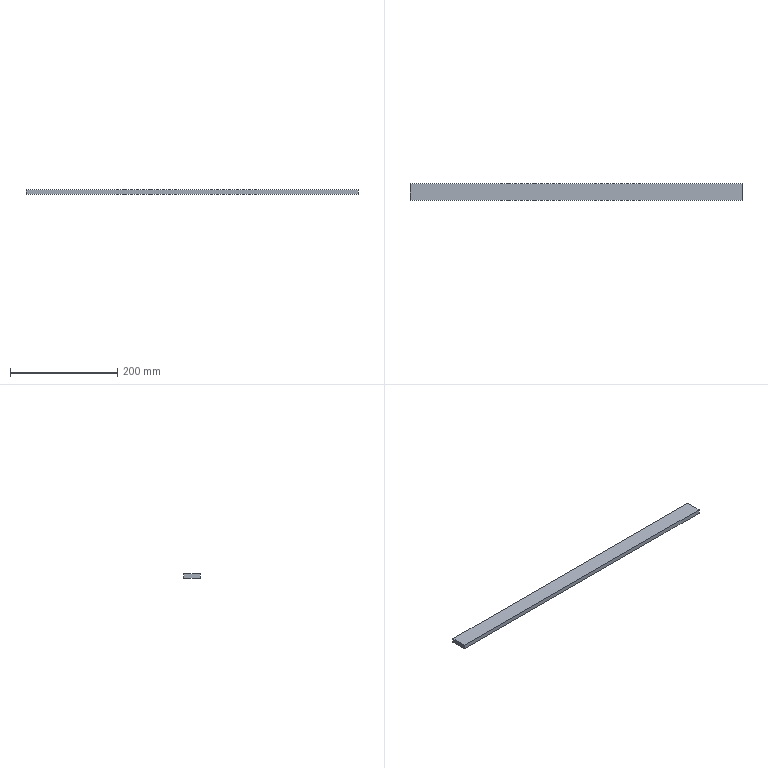Part | SolidWorks | features Extrusion 1 | 1 solid | 6 faces | box 620 x 30 x 8 mm | volume 148800 mm3 | plane 6
STEP:
#1=CARTESIAN_POINT('',(0.,30.,0.));
#2=VERTEX_POINT('',#1);
#3=CARTESIAN_POINT('',(0.,0.,0.));
#4=VERTEX_POINT('',#3);
#5=CARTESIAN_POINT('',(0.,0.,0.));
#6=DIRECTION('',(0.,-1.,0.));
#7=VECTOR('',#6,1000.);
#8=LINE('',#5,#7);
#9=EDGE_CURVE('',#2,#4,#8,.T.);
#10=ORIENTED_EDGE('',*,*,#9,.T.);
#11=CARTESIAN_POINT('',(0.,0.,8.));
#12=VERTEX_POINT('',#11);
#13=CARTESIAN_POINT('',(0.,0.,8.));
#14=DIRECTION('',(0.,0.,-1.));
#15=VECTOR('',#14,1000.);
#16=LINE('',#13,#15);
#17=EDGE_CURVE('',#12,#4,#16,.T.);
#18=ORIENTED_EDGE('',*,*,#17,.F.);
#19=CARTESIAN_POINT('',(0.,30.,8.));
#20=VERTEX_POINT('',#19);
#21=CARTESIAN_POINT('',(0.,0.,8.));
#22=DIRECTION('',(0.,-1.,0.));
#23=VECTOR('',#22,1000.);
#24=LINE('',#21,#23);
#25=EDGE_CURVE('',#20,#12,#24,.T.);
#26=ORIENTED_EDGE('',*,*,#25,.F.);
#27=CARTESIAN_POINT('',(0.,30.,8.));
#28=DIRECTION('',(0.,0.,-1.));
#29=VECTOR('',#28,1000.);
#30=LINE('',#27,#29);
#31=EDGE_CURVE('',#20,#2,#30,.T.);
#32=ORIENTED_EDGE('',*,*,#31,.T.);
#33=EDGE_LOOP('',(#10,#18,#26,#32));
#34=FACE_OUTER_BOUND('',#33,.T.);
#35=CARTESIAN_POINT('',(0.,0.,8.));
#36=DIRECTION('',(1.,0.,0.));
#37=DIRECTION('',(0.,0.,-1.));
#38=AXIS2_PLACEMENT_3D('',#35,#36,#37);
#39=PLANE('',#38);
#40=ADVANCED_FACE('',(#34),#39,.F.);
#41=CARTESIAN_POINT('',(620.,0.,0.));
#42=VERTEX_POINT('',#41);
#43=CARTESIAN_POINT('',(0.,0.,0.));
#44=DIRECTION('',(1.,0.,0.));
#45=VECTOR('',#44,1000.);
#46=LINE('',#43,#45);
#47=EDGE_CURVE('',#4,#42,#46,.T.);
#48=ORIENTED_EDGE('',*,*,#47,.T.);
#49=CARTESIAN_POINT('',(620.,0.,8.));
#50=VERTEX_POINT('',#49);
#51=CARTESIAN_POINT('',(620.,0.,8.));
#52=DIRECTION('',(0.,0.,-1.));
#53=VECTOR('',#52,1000.);
#54=LINE('',#51,#53);
#55=EDGE_CURVE('',#50,#42,#54,.T.);
#56=ORIENTED_EDGE('',*,*,#55,.F.);
#57=CARTESIAN_POINT('',(0.,0.,8.));
#58=DIRECTION('',(1.,0.,0.));
#59=VECTOR('',#58,1000.);
#60=LINE('',#57,#59);
#61=EDGE_CURVE('',#12,#50,#60,.T.);
#62=ORIENTED_EDGE('',*,*,#61,.F.);
#63=ORIENTED_EDGE('',*,*,#17,.T.);
#64=EDGE_LOOP('',(#48,#56,#62,#63));
#65=FACE_OUTER_BOUND('',#64,.T.);
#66=CARTESIAN_POINT('',(0.,0.,8.));
#67=DIRECTION('',(0.,1.,0.));
#68=DIRECTION('',(0.,0.,1.));
#69=AXIS2_PLACEMENT_3D('',#66,#67,#68);
#70=PLANE('',#69);
#71=ADVANCED_FACE('',(#65),#70,.F.);
#72=CARTESIAN_POINT('',(620.,30.,0.));
#73=VERTEX_POINT('',#72);
#74=CARTESIAN_POINT('',(620.,0.,0.));
#75=DIRECTION('',(0.,1.,0.));
#76=VECTOR('',#75,1000.);
#77=LINE('',#74,#76);
#78=EDGE_CURVE('',#42,#73,#77,.T.);
#79=ORIENTED_EDGE('',*,*,#78,.T.);
#80=CARTESIAN_POINT('',(620.,30.,8.));
#81=VERTEX_POINT('',#80);
#82=CARTESIAN_POINT('',(620.,30.,8.));
#83=DIRECTION('',(0.,0.,-1.));
#84=VECTOR('',#83,1000.);
#85=LINE('',#82,#84);
#86=EDGE_CURVE('',#81,#73,#85,.T.);
#87=ORIENTED_EDGE('',*,*,#86,.F.);
#88=CARTESIAN_POINT('',(620.,0.,8.));
#89=DIRECTION('',(0.,1.,0.));
#90=VECTOR('',#89,1000.);
#91=LINE('',#88,#90);
#92=EDGE_CURVE('',#50,#81,#91,.T.);
#93=ORIENTED_EDGE('',*,*,#92,.F.);
#94=ORIENTED_EDGE('',*,*,#55,.T.);
#95=EDGE_LOOP('',(#79,#87,#93,#94));
#96=FACE_OUTER_BOUND('',#95,.T.);
#97=CARTESIAN_POINT('',(620.,0.,8.));
#98=DIRECTION('',(-1.,0.,0.));
#99=DIRECTION('',(0.,0.,1.));
#100=AXIS2_PLACEMENT_3D('',#97,#98,#99);
#101=PLANE('',#100);
#102=ADVANCED_FACE('',(#96),#101,.F.);
#103=CARTESIAN_POINT('',(0.,30.,0.));
#104=DIRECTION('',(-1.,0.,0.));
#105=VECTOR('',#104,1000.);
#106=LINE('',#103,#105);
#107=EDGE_CURVE('',#73,#2,#106,.T.);
#108=ORIENTED_EDGE('',*,*,#107,.T.);
#109=ORIENTED_EDGE('',*,*,#31,.F.);
#110=CARTESIAN_POINT('',(0.,30.,8.));
#111=DIRECTION('',(-1.,0.,0.));
#112=VECTOR('',#111,1000.);
#113=LINE('',#110,#112);
#114=EDGE_CURVE('',#81,#20,#113,.T.);
#115=ORIENTED_EDGE('',*,*,#114,.F.);
#116=ORIENTED_EDGE('',*,*,#86,.T.);
#117=EDGE_LOOP('',(#108,#109,#115,#116));
#118=FACE_OUTER_BOUND('',#117,.T.);
#119=CARTESIAN_POINT('',(0.,30.,8.));
#120=DIRECTION('',(0.,-1.,0.));
#121=DIRECTION('',(0.,0.,-1.));
#122=AXIS2_PLACEMENT_3D('',#119,#120,#121);
#123=PLANE('',#122);
#124=ADVANCED_FACE('',(#118),#123,.F.);
#125=ORIENTED_EDGE('',*,*,#25,.T.);
#126=ORIENTED_EDGE('',*,*,#61,.T.);
#127=ORIENTED_EDGE('',*,*,#92,.T.);
#128=ORIENTED_EDGE('',*,*,#114,.T.);
#129=EDGE_LOOP('',(#125,#126,#127,#128));
#130=FACE_OUTER_BOUND('',#129,.T.);
#131=CARTESIAN_POINT('',(0.,30.,8.));
#132=DIRECTION('',(0.,0.,-1.));
#133=DIRECTION('',(-1.,0.,0.));
#134=AXIS2_PLACEMENT_3D('',#131,#132,#133);
#135=PLANE('',#134);
#136=ADVANCED_FACE('',(#130),#135,.F.);
#137=ORIENTED_EDGE('',*,*,#9,.F.);
#138=ORIENTED_EDGE('',*,*,#107,.F.);
#139=ORIENTED_EDGE('',*,*,#78,.F.);
#140=ORIENTED_EDGE('',*,*,#47,.F.);
#141=EDGE_LOOP('',(#137,#138,#139,#140));
#142=FACE_OUTER_BOUND('',#141,.T.);
#143=CARTESIAN_POINT('',(0.,30.,0.));
#144=DIRECTION('',(0.,0.,-1.));
#145=DIRECTION('',(-1.,0.,0.));
#146=AXIS2_PLACEMENT_3D('',#143,#144,#145);
#147=PLANE('',#146);
#148=ADVANCED_FACE('',(#142),#147,.T.);
#149=CLOSED_SHELL('',(#40,#71,#102,#124,#136,#148));
#150=MANIFOLD_SOLID_BREP('',#149);
#151=CARTESIAN_POINT('',(0.,0.,0.));
#152=DIRECTION('',(0.,0.,1.));
#153=DIRECTION('',(1.,0.,0.));
#154=AXIS2_PLACEMENT_3D('',#151,#152,#153);
#155=(LENGTH_UNIT()NAMED_UNIT(*)SI_UNIT(.MILLI.,.METRE.));
#156=UNCERTAINTY_MEASURE_WITH_UNIT(LENGTH_MEASURE(0.00001),#155,'','');
#157=(NAMED_UNIT(*)PLANE_ANGLE_UNIT()SI_UNIT($,.RADIAN.));
#158=(NAMED_UNIT(*)SI_UNIT($,.STERADIAN.)SOLID_ANGLE_UNIT());
#159=(GEOMETRIC_REPRESENTATION_CONTEXT(3)GLOBAL_UNCERTAINTY_ASSIGNED_CONTEXT((#156))GLOBAL_UNIT_ASSIGNED_CONTEXT((#155,#157,#158))REPRESENTATION_CONTEXT('',''));
#160=ADVANCED_BREP_SHAPE_REPRESENTATION('',(#150,#154),#159);